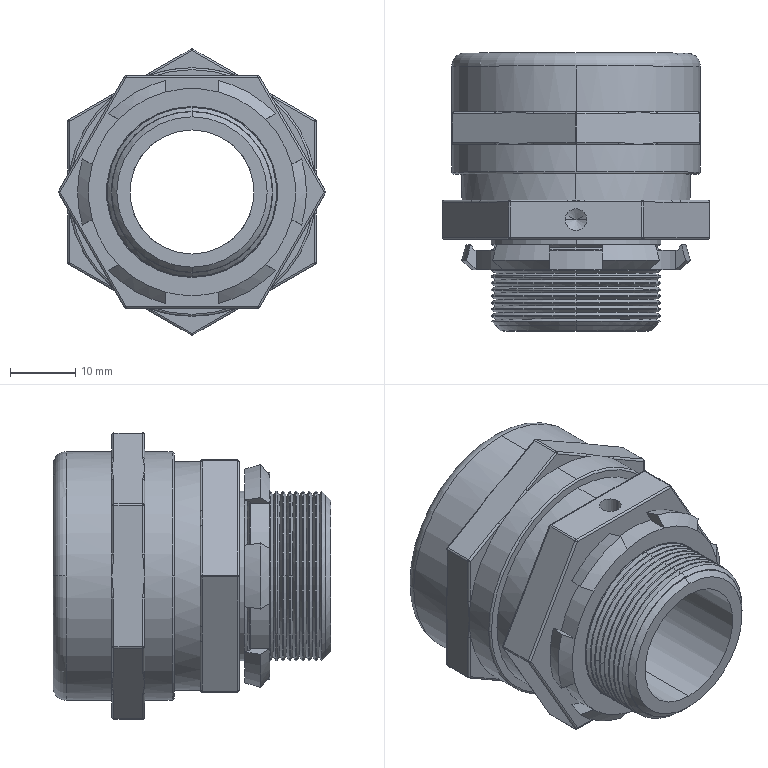Part | SolidWorks | features BaseBody 1 | 1 solid | 293 faces | box 40.899 x 42.5 x 43.786 mm | volume 24290 mm3 | cylinder 102 | cone 81 | plane 50 | spline 30 | sphere 24 | torus 6 | commonest cylinder face diameters 0.6 x55 26 x20 31.648 x7 26.163 x6 38 x4 3.3 x2